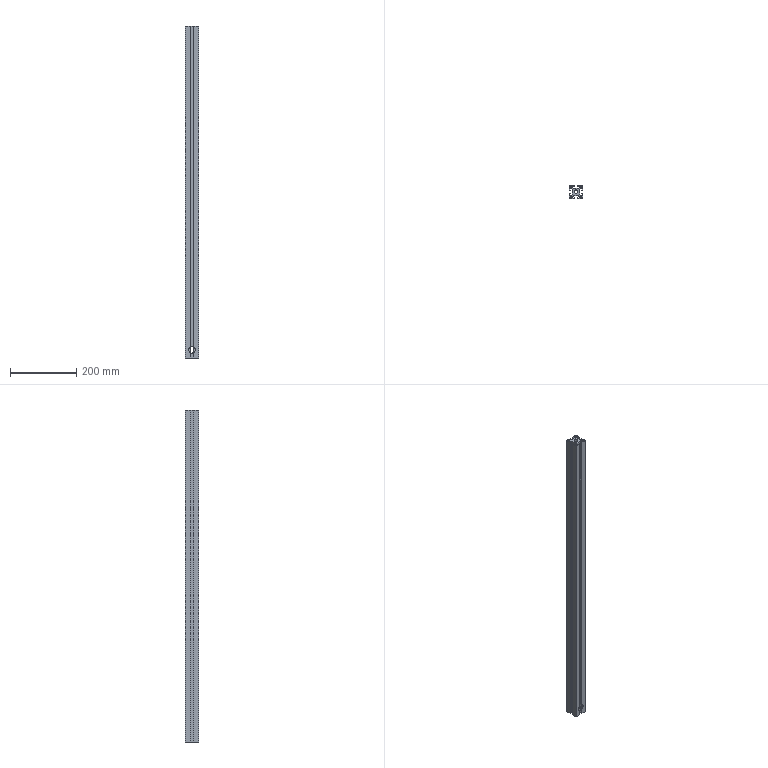Part | SolidWorks | features BaseBody 1 | 1 solid | 78 faces | box 40 x 40 x 1000 mm | volume 778881 mm3 | plane 62 | cylinder 16 | commonest cylinder face diameters 6 x8 20.5 x6 10.5 x2